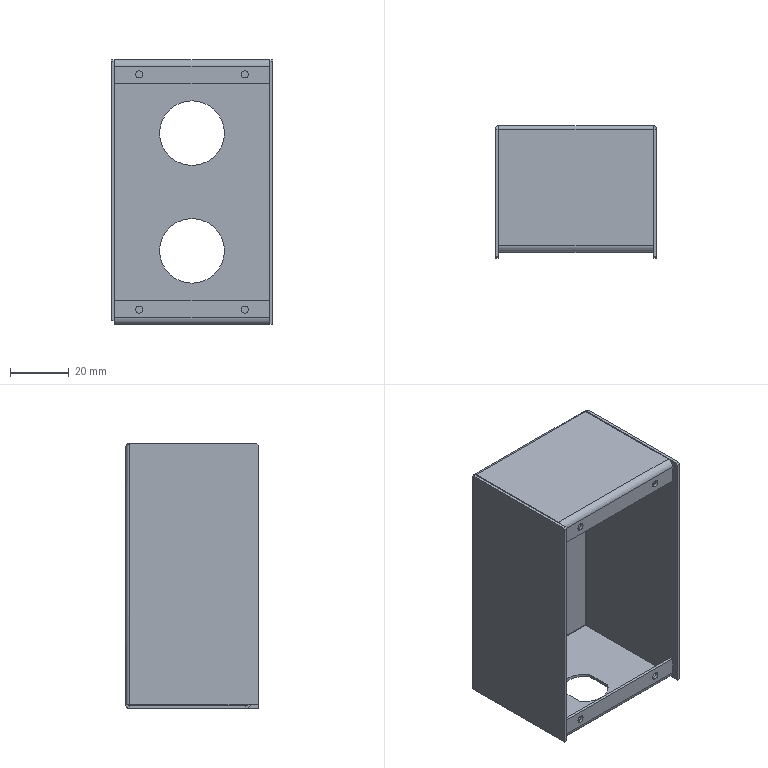Part | STEP file | Push button housing | 1 solid | 72 faces | box 55 x 45 x 90 mm | volume 16840 mm3 | plane 43 | cylinder 26 | spline 3 | commonest cylinder face diameters 2.5 x8 2.4 x6 0.4 x4 22 x4 4.4 x2 16 x2